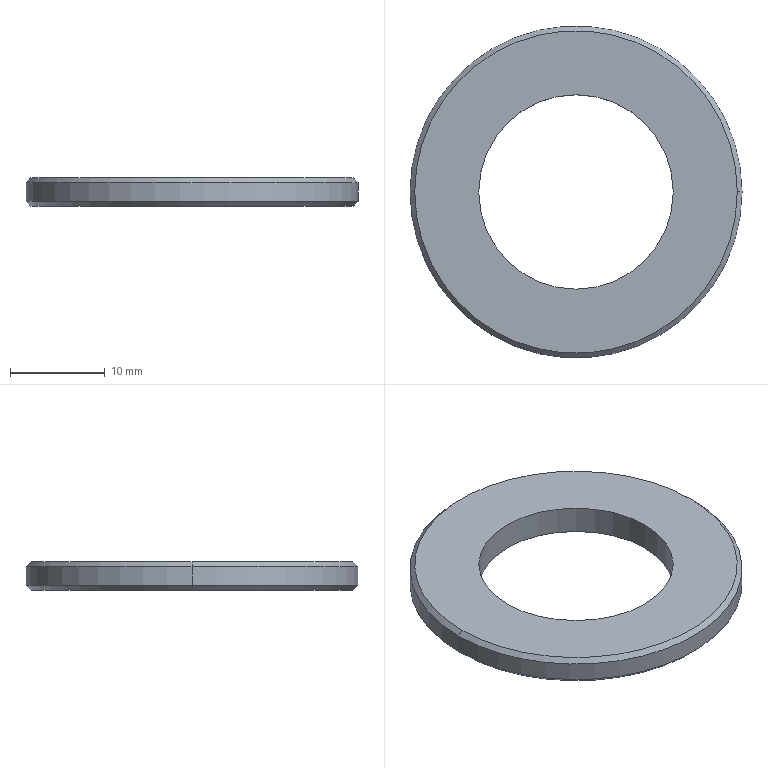Part | SolidWorks | features Chamfer 1, Extrusion 1 | 1 solid | 10 faces | box 35 x 35 x 3 mm | volume 1869 mm3 | cone 4 | cylinder 4 | plane 2 | commonest cylinder face diameters 20.5 x2 35 x2
STEP:
#1=CARTESIAN_POINT('',(17.,0.,3.));
#2=VERTEX_POINT('',#1);
#3=CARTESIAN_POINT('',(-17.,0.,3.));
#4=VERTEX_POINT('',#3);
#5=CARTESIAN_POINT('',(0.,0.,3.));
#6=DIRECTION('',(0.,0.,1.));
#7=DIRECTION('',(1.,0.,0.));
#8=AXIS2_PLACEMENT_3D('',#5,#6,#7);
#9=CIRCLE('',#8,17.);
#10=EDGE_CURVE('',#2,#4,#9,.T.);
#11=ORIENTED_EDGE('',*,*,#10,.F.);
#12=CARTESIAN_POINT('',(17.5,0.,2.5));
#13=VERTEX_POINT('',#12);
#14=CARTESIAN_POINT('',(17.,0.,3.));
#15=DIRECTION('',(0.7071,0.,-0.7071));
#16=VECTOR('',#15,1000.);
#17=LINE('',#14,#16);
#18=EDGE_CURVE('',#2,#13,#17,.T.);
#19=ORIENTED_EDGE('',*,*,#18,.T.);
#20=CARTESIAN_POINT('',(-17.5,0.,2.5));
#21=VERTEX_POINT('',#20);
#22=CARTESIAN_POINT('',(0.,0.,2.5));
#23=DIRECTION('',(0.,0.,-1.));
#24=DIRECTION('',(1.,0.,0.));
#25=AXIS2_PLACEMENT_3D('',#22,#23,#24);
#26=CIRCLE('',#25,17.5);
#27=EDGE_CURVE('',#21,#13,#26,.T.);
#28=ORIENTED_EDGE('',*,*,#27,.F.);
#29=CARTESIAN_POINT('',(-17.,0.,3.));
#30=DIRECTION('',(-0.7071,0.,-0.7071));
#31=VECTOR('',#30,1000.);
#32=LINE('',#29,#31);
#33=EDGE_CURVE('',#4,#21,#32,.T.);
#34=ORIENTED_EDGE('',*,*,#33,.F.);
#35=EDGE_LOOP('',(#11,#19,#28,#34));
#36=FACE_OUTER_BOUND('',#35,.T.);
#37=CARTESIAN_POINT('',(0.,0.,3.));
#38=DIRECTION('',(0.,0.,-1.));
#39=DIRECTION('',(-1.,0.,0.));
#40=AXIS2_PLACEMENT_3D('',#37,#38,#39);
#41=CONICAL_SURFACE('',#40,17.,0.7854);
#42=ADVANCED_FACE('',(#36),#41,.T.);
#43=CARTESIAN_POINT('',(-17.,0.,0.));
#44=VERTEX_POINT('',#43);
#45=CARTESIAN_POINT('',(17.,0.,0.));
#46=VERTEX_POINT('',#45);
#47=CARTESIAN_POINT('',(0.,0.,0.));
#48=DIRECTION('',(0.,0.,-1.));
#49=DIRECTION('',(1.,0.,0.));
#50=AXIS2_PLACEMENT_3D('',#47,#48,#49);
#51=CIRCLE('',#50,17.);
#52=EDGE_CURVE('',#44,#46,#51,.T.);
#53=ORIENTED_EDGE('',*,*,#52,.F.);
#54=CARTESIAN_POINT('',(-17.5,0.,0.5));
#55=VERTEX_POINT('',#54);
#56=CARTESIAN_POINT('',(-17.5,0.,0.5));
#57=DIRECTION('',(-0.7071,0.,0.7071));
#58=VECTOR('',#57,1000.);
#59=LINE('',#56,#58);
#60=EDGE_CURVE('',#44,#55,#59,.T.);
#61=ORIENTED_EDGE('',*,*,#60,.T.);
#62=CARTESIAN_POINT('',(17.5,0.,0.5));
#63=VERTEX_POINT('',#62);
#64=CARTESIAN_POINT('',(0.,0.,0.5));
#65=DIRECTION('',(0.,0.,1.));
#66=DIRECTION('',(1.,0.,0.));
#67=AXIS2_PLACEMENT_3D('',#64,#65,#66);
#68=CIRCLE('',#67,17.5);
#69=EDGE_CURVE('',#63,#55,#68,.T.);
#70=ORIENTED_EDGE('',*,*,#69,.F.);
#71=CARTESIAN_POINT('',(17.5,0.,0.5));
#72=DIRECTION('',(0.7071,0.,0.7071));
#73=VECTOR('',#72,1000.);
#74=LINE('',#71,#73);
#75=EDGE_CURVE('',#46,#63,#74,.T.);
#76=ORIENTED_EDGE('',*,*,#75,.F.);
#77=EDGE_LOOP('',(#53,#61,#70,#76));
#78=FACE_OUTER_BOUND('',#77,.T.);
#79=CARTESIAN_POINT('',(0.,0.,0.5));
#80=DIRECTION('',(0.,0.,1.));
#81=DIRECTION('',(1.,0.,0.));
#82=AXIS2_PLACEMENT_3D('',#79,#80,#81);
#83=CONICAL_SURFACE('',#82,17.5,0.7854);
#84=ADVANCED_FACE('',(#78),#83,.T.);
#85=CARTESIAN_POINT('',(-10.25,0.,3.));
#86=VERTEX_POINT('',#85);
#87=CARTESIAN_POINT('',(10.25,0.,3.));
#88=VERTEX_POINT('',#87);
#89=CARTESIAN_POINT('',(0.,0.,3.));
#90=DIRECTION('',(0.,0.,1.));
#91=DIRECTION('',(1.,0.,0.));
#92=AXIS2_PLACEMENT_3D('',#89,#90,#91);
#93=CIRCLE('',#92,10.25);
#94=EDGE_CURVE('',#86,#88,#93,.T.);
#95=ORIENTED_EDGE('',*,*,#94,.T.);
#96=CARTESIAN_POINT('',(10.25,0.,0.));
#97=VERTEX_POINT('',#96);
#98=CARTESIAN_POINT('',(10.25,0.,3.));
#99=DIRECTION('',(0.,0.,-1.));
#100=VECTOR('',#99,1000.);
#101=LINE('',#98,#100);
#102=EDGE_CURVE('',#88,#97,#101,.T.);
#103=ORIENTED_EDGE('',*,*,#102,.T.);
#104=CARTESIAN_POINT('',(-10.25,0.,0.));
#105=VERTEX_POINT('',#104);
#106=CARTESIAN_POINT('',(0.,0.,0.));
#107=DIRECTION('',(0.,0.,1.));
#108=DIRECTION('',(1.,0.,0.));
#109=AXIS2_PLACEMENT_3D('',#106,#107,#108);
#110=CIRCLE('',#109,10.25);
#111=EDGE_CURVE('',#105,#97,#110,.T.);
#112=ORIENTED_EDGE('',*,*,#111,.F.);
#113=CARTESIAN_POINT('',(-10.25,0.,3.));
#114=DIRECTION('',(0.,0.,-1.));
#115=VECTOR('',#114,1000.);
#116=LINE('',#113,#115);
#117=EDGE_CURVE('',#86,#105,#116,.T.);
#118=ORIENTED_EDGE('',*,*,#117,.F.);
#119=EDGE_LOOP('',(#95,#103,#112,#118));
#120=FACE_OUTER_BOUND('',#119,.T.);
#121=CARTESIAN_POINT('',(0.,0.,3.));
#122=DIRECTION('',(0.,0.,-1.));
#123=DIRECTION('',(-1.,0.,0.));
#124=AXIS2_PLACEMENT_3D('',#121,#122,#123);
#125=CYLINDRICAL_SURFACE('',#124,10.25);
#126=ADVANCED_FACE('',(#120),#125,.F.);
#127=ORIENTED_EDGE('',*,*,#27,.T.);
#128=CARTESIAN_POINT('',(17.5,0.,3.));
#129=DIRECTION('',(0.,0.,-1.));
#130=VECTOR('',#129,1000.);
#131=LINE('',#128,#130);
#132=EDGE_CURVE('',#13,#63,#131,.T.);
#133=ORIENTED_EDGE('',*,*,#132,.T.);
#134=ORIENTED_EDGE('',*,*,#69,.T.);
#135=CARTESIAN_POINT('',(-17.5,0.,3.));
#136=DIRECTION('',(0.,0.,-1.));
#137=VECTOR('',#136,1000.);
#138=LINE('',#135,#137);
#139=EDGE_CURVE('',#21,#55,#138,.T.);
#140=ORIENTED_EDGE('',*,*,#139,.F.);
#141=EDGE_LOOP('',(#127,#133,#134,#140));
#142=FACE_OUTER_BOUND('',#141,.T.);
#143=CARTESIAN_POINT('',(0.,0.,3.));
#144=DIRECTION('',(0.,0.,-1.));
#145=DIRECTION('',(-1.,0.,0.));
#146=AXIS2_PLACEMENT_3D('',#143,#144,#145);
#147=CYLINDRICAL_SURFACE('',#146,17.5);
#148=ADVANCED_FACE('',(#142),#147,.T.);
#149=CARTESIAN_POINT('',(0.,0.,3.));
#150=DIRECTION('',(0.,0.,1.));
#151=DIRECTION('',(1.,0.,0.));
#152=AXIS2_PLACEMENT_3D('',#149,#150,#151);
#153=CIRCLE('',#152,17.);
#154=EDGE_CURVE('',#4,#2,#153,.T.);
#155=ORIENTED_EDGE('',*,*,#154,.T.);
#156=ORIENTED_EDGE('',*,*,#10,.T.);
#157=EDGE_LOOP('',(#155,#156));
#158=FACE_OUTER_BOUND('',#157,.T.);
#159=ORIENTED_EDGE('',*,*,#94,.F.);
#160=CARTESIAN_POINT('',(0.,0.,3.));
#161=DIRECTION('',(0.,0.,1.));
#162=DIRECTION('',(1.,0.,0.));
#163=AXIS2_PLACEMENT_3D('',#160,#161,#162);
#164=CIRCLE('',#163,10.25);
#165=EDGE_CURVE('',#88,#86,#164,.T.);
#166=ORIENTED_EDGE('',*,*,#165,.F.);
#167=EDGE_LOOP('',(#159,#166));
#168=FACE_BOUND('',#167,.T.);
#169=CARTESIAN_POINT('',(0.,0.,3.));
#170=DIRECTION('',(0.,0.,1.));
#171=DIRECTION('',(1.,0.,0.));
#172=AXIS2_PLACEMENT_3D('',#169,#170,#171);
#173=PLANE('',#172);
#174=ADVANCED_FACE('',(#158,#168),#173,.T.);
#175=CARTESIAN_POINT('',(0.,0.,0.));
#176=DIRECTION('',(0.,0.,-1.));
#177=DIRECTION('',(1.,0.,0.));
#178=AXIS2_PLACEMENT_3D('',#175,#176,#177);
#179=CIRCLE('',#178,17.);
#180=EDGE_CURVE('',#46,#44,#179,.T.);
#181=ORIENTED_EDGE('',*,*,#180,.T.);
#182=ORIENTED_EDGE('',*,*,#52,.T.);
#183=EDGE_LOOP('',(#181,#182));
#184=FACE_OUTER_BOUND('',#183,.T.);
#185=ORIENTED_EDGE('',*,*,#111,.T.);
#186=CARTESIAN_POINT('',(0.,0.,0.));
#187=DIRECTION('',(0.,0.,1.));
#188=DIRECTION('',(1.,0.,0.));
#189=AXIS2_PLACEMENT_3D('',#186,#187,#188);
#190=CIRCLE('',#189,10.25);
#191=EDGE_CURVE('',#97,#105,#190,.T.);
#192=ORIENTED_EDGE('',*,*,#191,.T.);
#193=EDGE_LOOP('',(#185,#192));
#194=FACE_BOUND('',#193,.T.);
#195=CARTESIAN_POINT('',(0.,0.,0.));
#196=DIRECTION('',(0.,0.,1.));
#197=DIRECTION('',(1.,0.,0.));
#198=AXIS2_PLACEMENT_3D('',#195,#196,#197);
#199=PLANE('',#198);
#200=ADVANCED_FACE('',(#184,#194),#199,.F.);
#201=ORIENTED_EDGE('',*,*,#132,.F.);
#202=CARTESIAN_POINT('',(0.,0.,2.5));
#203=DIRECTION('',(0.,0.,-1.));
#204=DIRECTION('',(1.,0.,0.));
#205=AXIS2_PLACEMENT_3D('',#202,#203,#204);
#206=CIRCLE('',#205,17.5);
#207=EDGE_CURVE('',#13,#21,#206,.T.);
#208=ORIENTED_EDGE('',*,*,#207,.T.);
#209=ORIENTED_EDGE('',*,*,#139,.T.);
#210=CARTESIAN_POINT('',(0.,0.,0.5));
#211=DIRECTION('',(0.,0.,1.));
#212=DIRECTION('',(1.,0.,0.));
#213=AXIS2_PLACEMENT_3D('',#210,#211,#212);
#214=CIRCLE('',#213,17.5);
#215=EDGE_CURVE('',#55,#63,#214,.T.);
#216=ORIENTED_EDGE('',*,*,#215,.T.);
#217=EDGE_LOOP('',(#201,#208,#209,#216));
#218=FACE_OUTER_BOUND('',#217,.T.);
#219=CARTESIAN_POINT('',(0.,0.,3.));
#220=DIRECTION('',(0.,0.,-1.));
#221=DIRECTION('',(-1.,0.,0.));
#222=AXIS2_PLACEMENT_3D('',#219,#220,#221);
#223=CYLINDRICAL_SURFACE('',#222,17.5);
#224=ADVANCED_FACE('',(#218),#223,.T.);
#225=ORIENTED_EDGE('',*,*,#102,.F.);
#226=ORIENTED_EDGE('',*,*,#165,.T.);
#227=ORIENTED_EDGE('',*,*,#117,.T.);
#228=ORIENTED_EDGE('',*,*,#191,.F.);
#229=EDGE_LOOP('',(#225,#226,#227,#228));
#230=FACE_OUTER_BOUND('',#229,.T.);
#231=CARTESIAN_POINT('',(0.,0.,3.));
#232=DIRECTION('',(0.,0.,-1.));
#233=DIRECTION('',(-1.,0.,0.));
#234=AXIS2_PLACEMENT_3D('',#231,#232,#233);
#235=CYLINDRICAL_SURFACE('',#234,10.25);
#236=ADVANCED_FACE('',(#230),#235,.F.);
#237=ORIENTED_EDGE('',*,*,#60,.F.);
#238=ORIENTED_EDGE('',*,*,#180,.F.);
#239=ORIENTED_EDGE('',*,*,#75,.T.);
#240=ORIENTED_EDGE('',*,*,#215,.F.);
#241=EDGE_LOOP('',(#237,#238,#239,#240));
#242=FACE_OUTER_BOUND('',#241,.T.);
#243=CARTESIAN_POINT('',(0.,0.,0.5));
#244=DIRECTION('',(0.,0.,1.));
#245=DIRECTION('',(1.,0.,0.));
#246=AXIS2_PLACEMENT_3D('',#243,#244,#245);
#247=CONICAL_SURFACE('',#246,17.5,0.7854);
#248=ADVANCED_FACE('',(#242),#247,.T.);
#249=ORIENTED_EDGE('',*,*,#18,.F.);
#250=ORIENTED_EDGE('',*,*,#154,.F.);
#251=ORIENTED_EDGE('',*,*,#33,.T.);
#252=ORIENTED_EDGE('',*,*,#207,.F.);
#253=EDGE_LOOP('',(#249,#250,#251,#252));
#254=FACE_OUTER_BOUND('',#253,.T.);
#255=CARTESIAN_POINT('',(0.,0.,3.));
#256=DIRECTION('',(0.,0.,-1.));
#257=DIRECTION('',(-1.,0.,0.));
#258=AXIS2_PLACEMENT_3D('',#255,#256,#257);
#259=CONICAL_SURFACE('',#258,17.,0.7854);
#260=ADVANCED_FACE('',(#254),#259,.T.);
#261=CLOSED_SHELL('',(#42,#84,#126,#148,#174,#200,#224,#236,#248,#260));
#262=MANIFOLD_SOLID_BREP('',#261);
#263=CARTESIAN_POINT('',(0.,0.,0.));
#264=DIRECTION('',(0.,0.,1.));
#265=DIRECTION('',(1.,0.,0.));
#266=AXIS2_PLACEMENT_3D('',#263,#264,#265);
#267=(LENGTH_UNIT()NAMED_UNIT(*)SI_UNIT(.MILLI.,.METRE.));
#268=UNCERTAINTY_MEASURE_WITH_UNIT(LENGTH_MEASURE(0.00001),#267,'','');
#269=(NAMED_UNIT(*)PLANE_ANGLE_UNIT()SI_UNIT($,.RADIAN.));
#270=(NAMED_UNIT(*)SI_UNIT($,.STERADIAN.)SOLID_ANGLE_UNIT());
#271=(GEOMETRIC_REPRESENTATION_CONTEXT(3)GLOBAL_UNCERTAINTY_ASSIGNED_CONTEXT((#268))GLOBAL_UNIT_ASSIGNED_CONTEXT((#267,#269,#270))REPRESENTATION_CONTEXT('',''));
#272=ADVANCED_BREP_SHAPE_REPRESENTATION('',(#262,#266),#271);